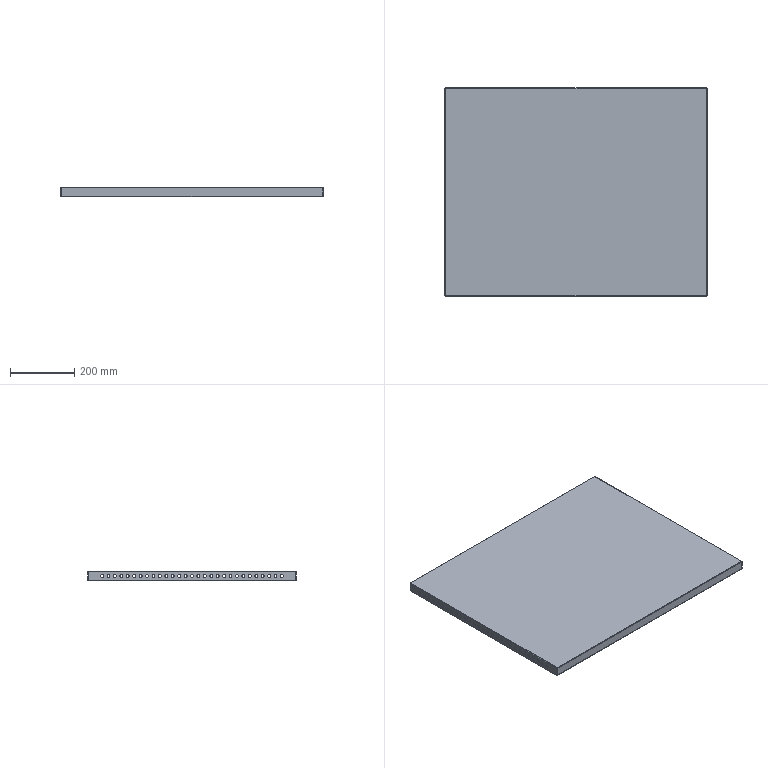Part | SolidWorks | features EdgeFlange 2, FlatPattern 1, ICE 1, SMBaseFlange 1, SheetMetal 1 | 1 solid | 186 faces | box 816 x 650 x 30 mm | volume 1268651 mm3 | cylinder 132 | plane 38 | spline 16 | commonest cylinder face diameters 9 x116 0.2 x8 4.2 x8